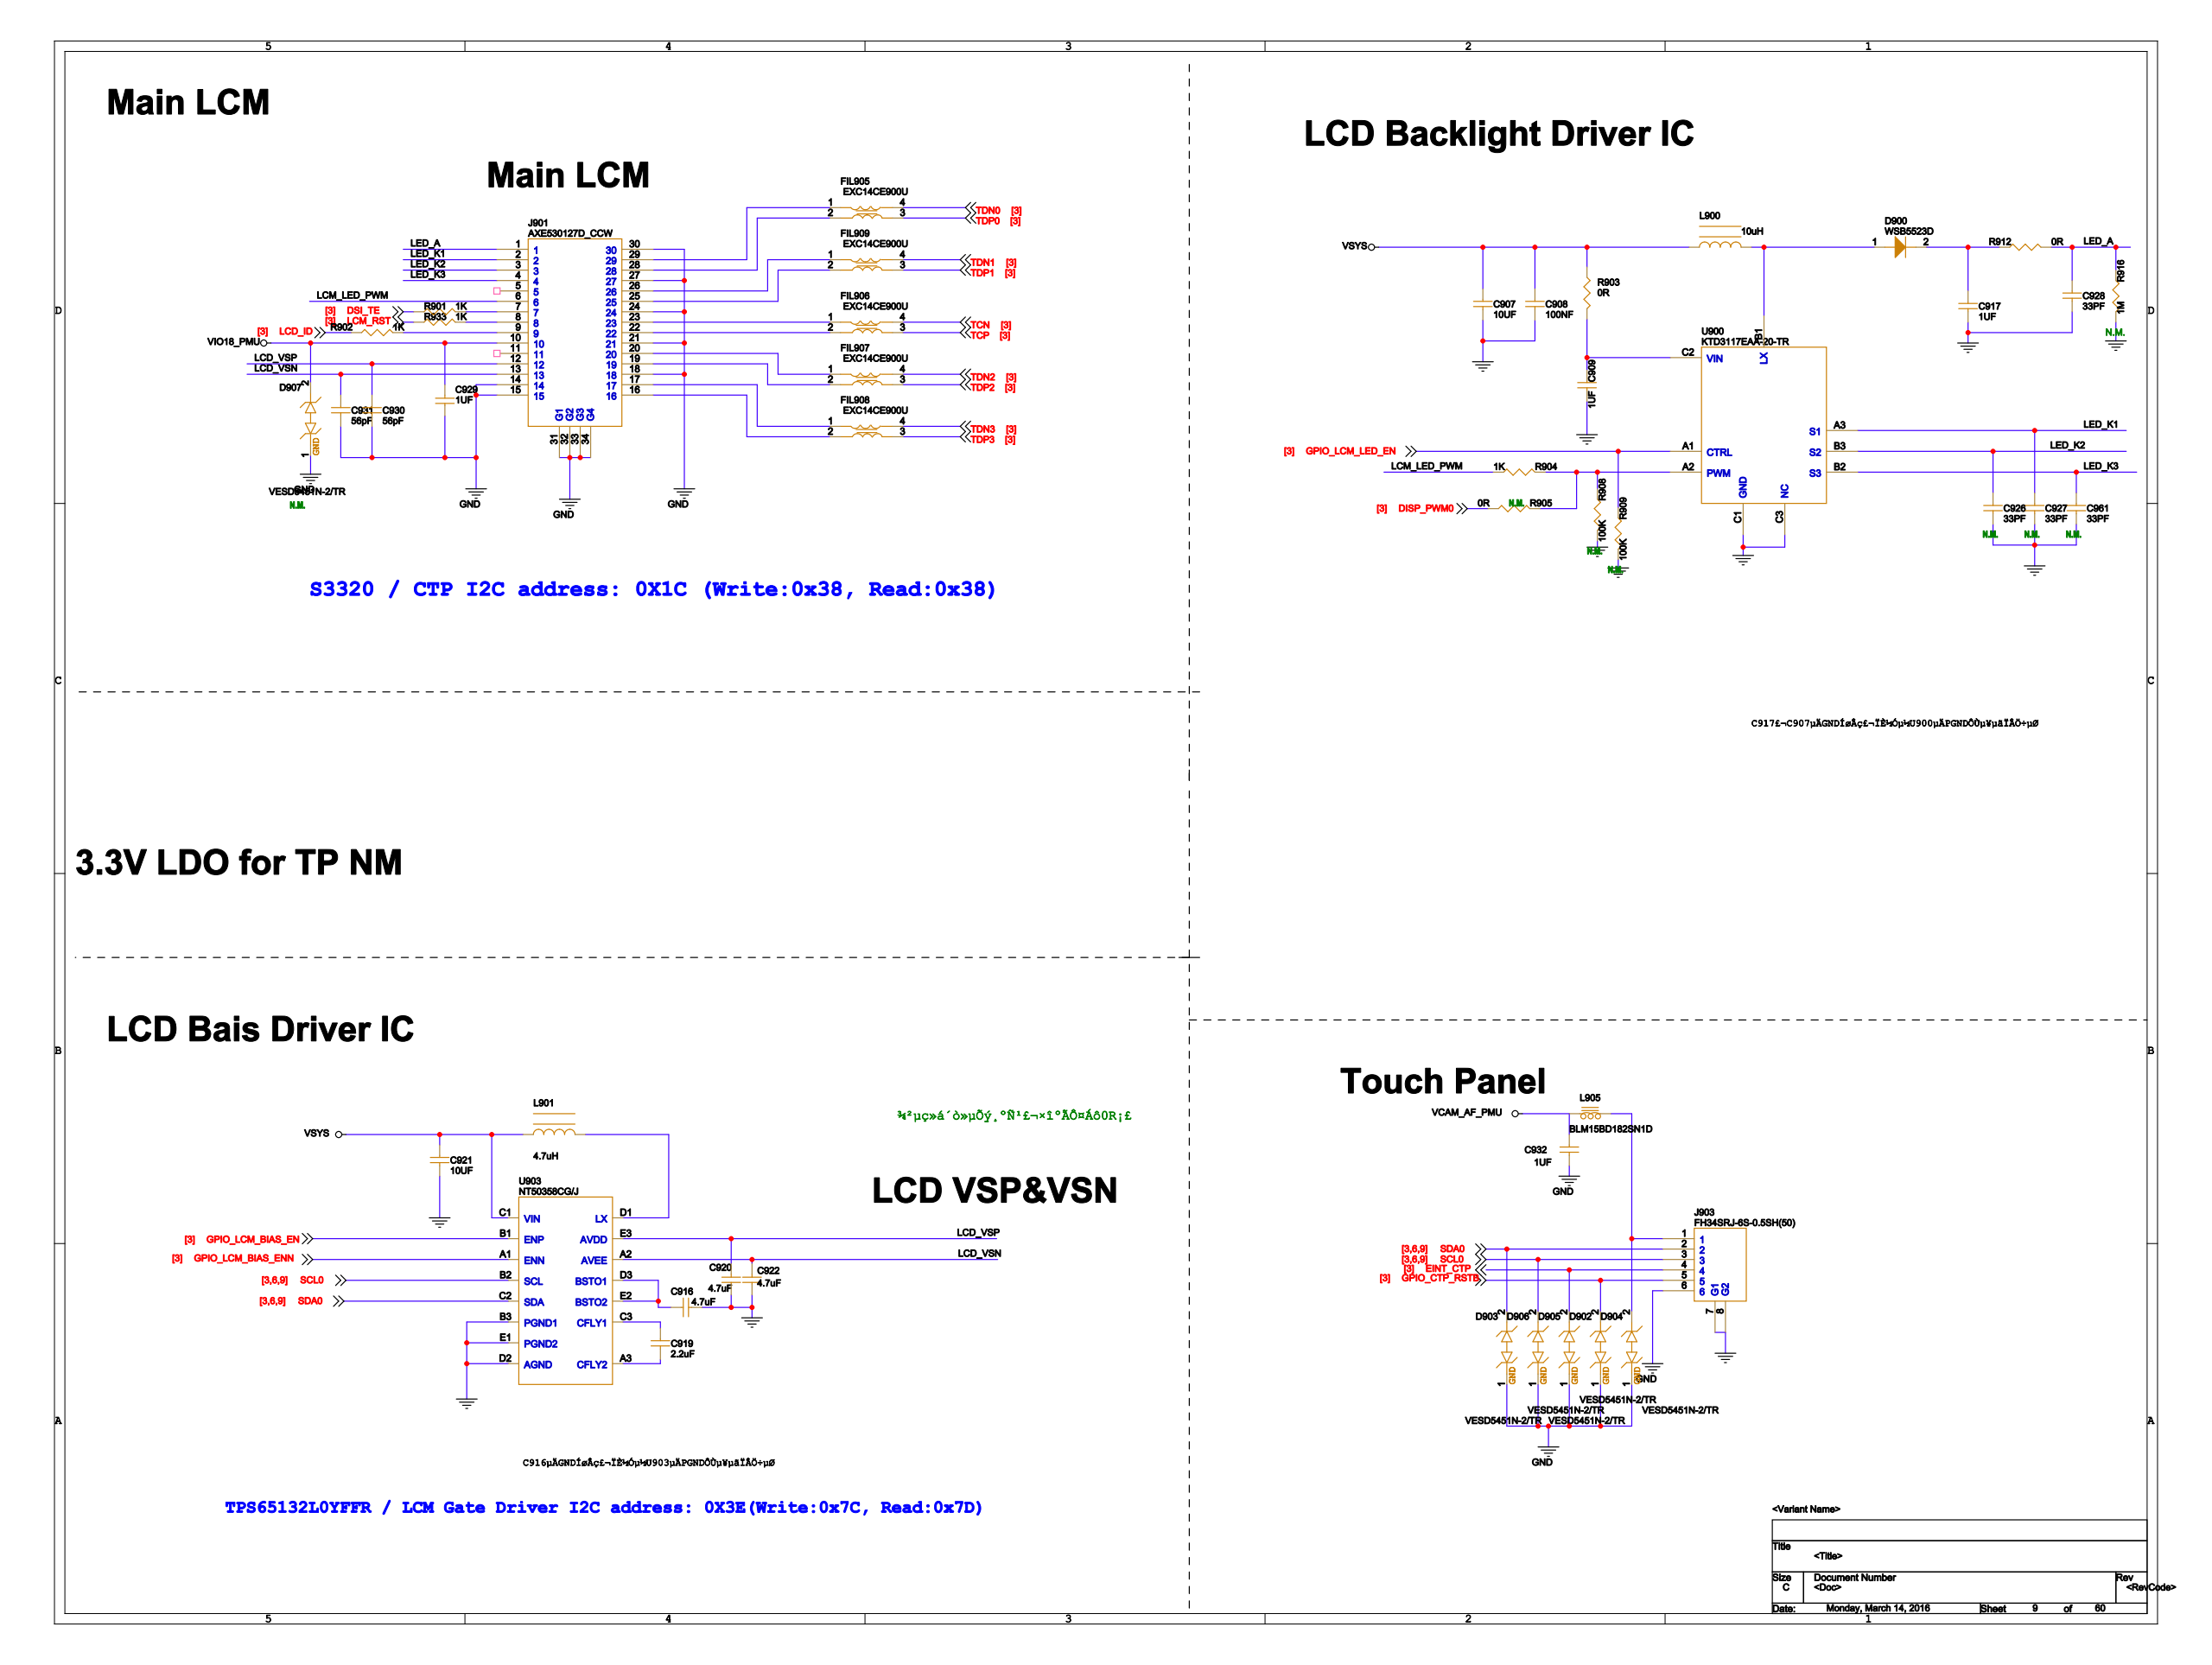Circuit board | Cadence Allegro | 1088 parts | 793 nets | one sheet of the schematic
Parts on this sheet (reference | value | footprint):
C907 | 10UF | 0402-BIG
C908 | 100NF | C0201
C909 | 1UF | C0201
C916 | 4.7uF | 0402-BIG
C917 | 1UF | C0603
C919 | 2.2uF | 0603-BIG
C920 | 4.7uF | 0402-BIG
C921 | 10UF | 0402-BIG
C922 | 4.7uF | 0402-BIG
C926
C927
C928 | 33PF | C0201
C929 | 1UF | C0201
C930 | 56pF | C0201
C931 | 56pF | C0201
C932 | 1UF | C0201
C961
D900 | WSB5523D | FBP1608-WSB5524D
D902 | VESD5451N-2/TR | DFN1006-2
D903 | VESD5451N-2/TR | DFN1006-2
D904 | VESD5451N-2/TR | DFN1006-2
D905 | VESD5451N-2/TR | DFN1006-2
D906 | VESD5451N-2/TR | DFN1006-2
D907
FIL905 | EXC14CE900U | EXC14CE900U
FIL906 | EXC14CE900U | EXC14CE900U
FIL907 | EXC14CE900U | EXC14CE900U
FIL908 | EXC14CE900U | EXC14CE900U
FIL909 | EXC14CE900U | EXC14CE900U
J901 | AXE530127D_CCW | BTB_AXE530124_CCW
J903 | FH34SRJ-6S-0.5SH(50) | ZIF_FH34SRJ-6S-0_5SH_50
L900 | 10uH | L2520_VLS252010HBX-1
L901 | 4.7uH | L2016_VLS201610HBX-1
L905 | BLM15BD182SN1D | BLM15BD182SN1D
R901 | 1K | R0201
R902 | 1K | R0201
R903 | 0R | R0201
R904 | 1K | R0201
R905
R908
R909
R912 | 0R | R0402
R916
R933 | 1K | R0201
U900 | KTD3117EAA-20-TR | WLCSP9_1P2X1P2X0P755_0P4
U903 | NT50358CG/J | CSP15_1P36X2P26X0P78_0P4
Nets of these parts (net: part-pin ...):
GND: C907-2 C908-2 C909-2 C916-2 C917-2 C920-1 C921-2 C922-1 C926-2 C927-2 C928-2 C929-1 C930-2 C931-2 C932-2 C961-2 D902-1 D903-1 D904-1 D905-1 D906-1 D907-1 J903-6 J903-7 J903-8 R908-2 R909-2 R916-2 U900-C1 U900-C3 U903-B3 U903-D2 U903-E1 J901-14 J901-15 J901-18 J901-21 J901-24 J901-27 J901-30 J901-31 J901-32 J901-33 J901-34
VSYS: C907-1 C908-1 C921-1 L900-1 L901-1 R903-1 U903-C1
N34332726: L901-2 U903-D1
N31647745: D900-1 L900-2 U900-B1
DISP_PWM0: R905-1
LCD_ID: R902-1
DSI_TE: R901-1
LCM_RST: R933-1
TCN: FIL906-4
TCP: FIL906-3
TDN0: FIL905-4
TDN1: FIL909-4
TDN2: FIL907-4
TDN3: FIL908-4
TDP0: FIL905-3
TDP1: FIL909-3
TDP2: FIL907-3
TDP3: FIL908-3
EINT_CTP: D905-2 J903-4
GPIO_CTP_RSTB: D902-2 J903-5
GPIO_LCM_LED_EN: R909-1 U900-A1
GPIO_LCM_BIAS_EN: U903-B1
SCL0: D906-2 J903-3 U903-B2
SDA0: D903-2 J903-2 U903-C2
GPIO_LCM_BIAS_ENN: U903-A1
VIO18_PMU: C929-2 D907-2 J901-10
N31647747: R904-2 R905-2 R908-1 U900-A2
LED_K1: C927-1 U900-A3 J901-2
LED_K2: C926-1 U900-B3 J901-3
LED_K3: C961-1 U900-B2 J901-4
N31647765: C909-1 R903-2 U900-C2
N33341414: FIL905-1 J901-29
N33341408: FIL905-2 J901-28
N33341394: FIL906-1 J901-23
N33341392: FIL906-2 J901-22
N33341384: FIL907-1 J901-20
N33341380: FIL907-2 J901-19
N33341368: FIL908-1 J901-17
N33341372: FIL908-2 J901-16
N33341400: FIL909-1 J901-26
N33341396: FIL909-2 J901-25
LCD_VSP: C920-2 C930-1 U903-E3 J901-12
LCD_VSN: C922-2 C931-1 U903-A2 J901-13
N34333565: C916-1 U903-D3 U903-E2
N34334229: C919-1 U903-C3
N34334236: C919-2 U903-A3
N33341777: D904-2 J903-1 L905-2
VCAM_AF_PMU: C932-1 L905-1
LED_A: C928-1 R912-2 R916-1 J901-1
N31647739: C917-1 D900-2 R912-1
LCM_LED_PWM: R904-1 J901-6
N33341275: R901-2 J901-7
N33341277: R933-2 J901-8
N33341279: R902-2 J901-9